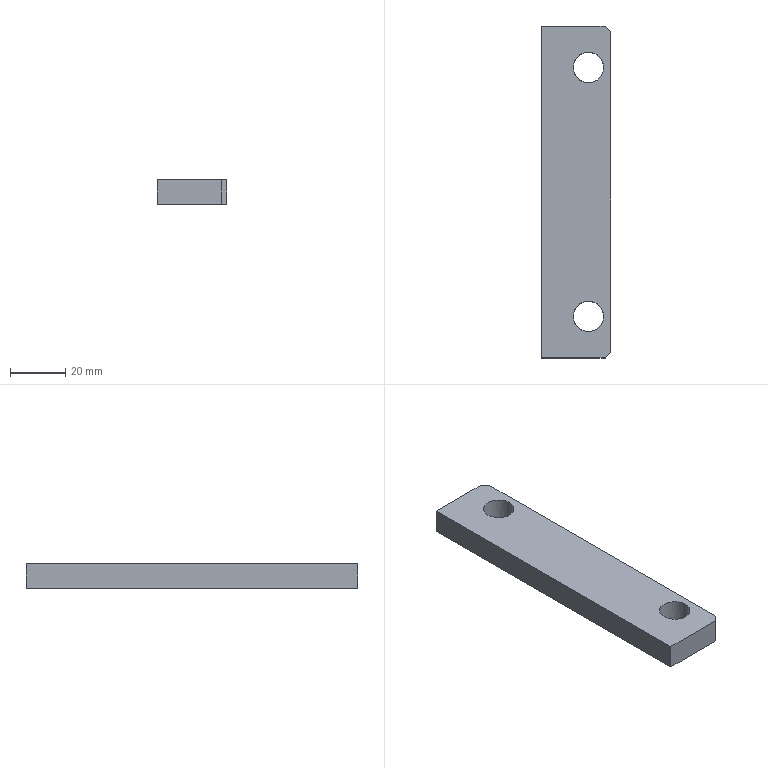Part | NX | features solid 2 | 1 solid | 10 faces | box 25 x 120 x 9 mm | volume 25253 mm3 | plane 8 | cylinder 2 | commonest cylinder face diameters 11 x2
STEP:
#1=CARTESIAN_POINT('',(59.5,685.,-99.));
#2=VERTEX_POINT('',#1);
#3=CARTESIAN_POINT('',(54.,685.,-99.));
#4=DIRECTION('',(0.,0.,1.));
#5=DIRECTION('',(1.,0.,0.));
#6=AXIS2_PLACEMENT_3D('',#3,#4,#5);
#7=CIRCLE('',#6,5.5);
#8=EDGE_CURVE('',#2,#2,#7,.F.);
#9=ORIENTED_EDGE('',*,*,#8,.T.);
#10=EDGE_LOOP('',(#9));
#11=FACE_BOUND('',#10,.T.);
#12=CARTESIAN_POINT('',(59.5,595.,-99.));
#13=VERTEX_POINT('',#12);
#14=CARTESIAN_POINT('',(54.,595.,-99.));
#15=DIRECTION('',(0.,0.,1.));
#16=DIRECTION('',(1.,0.,0.));
#17=AXIS2_PLACEMENT_3D('',#14,#15,#16);
#18=CIRCLE('',#17,5.5);
#19=EDGE_CURVE('',#13,#13,#18,.F.);
#20=ORIENTED_EDGE('',*,*,#19,.T.);
#21=EDGE_LOOP('',(#20));
#22=FACE_BOUND('',#21,.T.);
#23=CARTESIAN_POINT('',(62.,698.,-99.));
#24=VERTEX_POINT('',#23);
#25=CARTESIAN_POINT('',(62.,582.,-99.));
#26=VERTEX_POINT('',#25);
#27=CARTESIAN_POINT('',(62.,640.,-99.));
#28=DIRECTION('',(0.,-1.,0.));
#29=VECTOR('',#28,1000.);
#30=LINE('',#27,#29);
#31=EDGE_CURVE('',#24,#26,#30,.T.);
#32=ORIENTED_EDGE('',*,*,#31,.F.);
#33=CARTESIAN_POINT('',(60.,700.,-99.));
#34=VERTEX_POINT('',#33);
#35=CARTESIAN_POINT('',(84.75,675.25,-99.));
#36=DIRECTION('',(0.7071,-0.7071,0.));
#37=VECTOR('',#36,1000.);
#38=LINE('',#35,#37);
#39=EDGE_CURVE('',#24,#34,#38,.F.);
#40=ORIENTED_EDGE('',*,*,#39,.T.);
#41=CARTESIAN_POINT('',(37.,700.,-99.));
#42=VERTEX_POINT('',#41);
#43=CARTESIAN_POINT('',(49.5,700.,-99.));
#44=DIRECTION('',(1.,0.,0.));
#45=VECTOR('',#44,1000.);
#46=LINE('',#43,#45);
#47=EDGE_CURVE('',#42,#34,#46,.T.);
#48=ORIENTED_EDGE('',*,*,#47,.F.);
#49=CARTESIAN_POINT('',(37.,580.,-99.));
#50=VERTEX_POINT('',#49);
#51=CARTESIAN_POINT('',(37.,640.,-99.));
#52=DIRECTION('',(0.,1.,0.));
#53=VECTOR('',#52,1000.);
#54=LINE('',#51,#53);
#55=EDGE_CURVE('',#50,#42,#54,.T.);
#56=ORIENTED_EDGE('',*,*,#55,.F.);
#57=CARTESIAN_POINT('',(60.,580.,-99.));
#58=VERTEX_POINT('',#57);
#59=CARTESIAN_POINT('',(49.5,580.,-99.));
#60=DIRECTION('',(-1.,0.,0.));
#61=VECTOR('',#60,1000.);
#62=LINE('',#59,#61);
#63=EDGE_CURVE('',#58,#50,#62,.T.);
#64=ORIENTED_EDGE('',*,*,#63,.F.);
#65=CARTESIAN_POINT('',(84.75,604.75,-99.));
#66=DIRECTION('',(-0.7071,-0.7071,0.));
#67=VECTOR('',#66,1000.);
#68=LINE('',#65,#67);
#69=EDGE_CURVE('',#58,#26,#68,.F.);
#70=ORIENTED_EDGE('',*,*,#69,.T.);
#71=EDGE_LOOP('',(#32,#40,#48,#56,#64,#70));
#72=FACE_BOUND('',#71,.T.);
#73=CARTESIAN_POINT('',(49.5,640.,-99.));
#74=DIRECTION('',(0.,0.,1.));
#75=DIRECTION('',(0.,1.,0.));
#76=AXIS2_PLACEMENT_3D('',#73,#74,#75);
#77=PLANE('',#76);
#78=ADVANCED_FACE('',(#11,#22,#72),#77,.T.);
#79=CARTESIAN_POINT('',(62.,582.,-108.));
#80=VERTEX_POINT('',#79);
#81=CARTESIAN_POINT('',(62.,698.,-108.));
#82=VERTEX_POINT('',#81);
#83=CARTESIAN_POINT('',(62.,640.,-108.));
#84=DIRECTION('',(0.,1.,0.));
#85=VECTOR('',#84,1000.);
#86=LINE('',#83,#85);
#87=EDGE_CURVE('',#80,#82,#86,.T.);
#88=ORIENTED_EDGE('',*,*,#87,.T.);
#89=CARTESIAN_POINT('',(62.,698.,-108.));
#90=DIRECTION('',(0.,0.,1.));
#91=VECTOR('',#90,1000.);
#92=LINE('',#89,#91);
#93=EDGE_CURVE('',#82,#24,#92,.T.);
#94=ORIENTED_EDGE('',*,*,#93,.T.);
#95=ORIENTED_EDGE('',*,*,#31,.T.);
#96=CARTESIAN_POINT('',(62.,582.,-108.));
#97=DIRECTION('',(0.,0.,-1.));
#98=VECTOR('',#97,1000.);
#99=LINE('',#96,#98);
#100=EDGE_CURVE('',#26,#80,#99,.T.);
#101=ORIENTED_EDGE('',*,*,#100,.T.);
#102=EDGE_LOOP('',(#88,#94,#95,#101));
#103=FACE_BOUND('',#102,.T.);
#104=CARTESIAN_POINT('',(62.,640.,-108.));
#105=DIRECTION('',(1.,0.,0.));
#106=DIRECTION('',(0.,0.,-1.));
#107=AXIS2_PLACEMENT_3D('',#104,#105,#106);
#108=PLANE('',#107);
#109=ADVANCED_FACE('',(#103),#108,.T.);
#110=CARTESIAN_POINT('',(37.,580.,-108.));
#111=VERTEX_POINT('',#110);
#112=CARTESIAN_POINT('',(60.,580.,-108.));
#113=VERTEX_POINT('',#112);
#114=CARTESIAN_POINT('',(49.5,580.,-108.));
#115=DIRECTION('',(1.,0.,0.));
#116=VECTOR('',#115,1000.);
#117=LINE('',#114,#116);
#118=EDGE_CURVE('',#111,#113,#117,.T.);
#119=ORIENTED_EDGE('',*,*,#118,.T.);
#120=CARTESIAN_POINT('',(60.,580.,-108.));
#121=DIRECTION('',(0.,0.,1.));
#122=VECTOR('',#121,1000.);
#123=LINE('',#120,#122);
#124=EDGE_CURVE('',#113,#58,#123,.T.);
#125=ORIENTED_EDGE('',*,*,#124,.T.);
#126=ORIENTED_EDGE('',*,*,#63,.T.);
#127=CARTESIAN_POINT('',(37.,580.,-108.));
#128=DIRECTION('',(0.,0.,1.));
#129=VECTOR('',#128,1000.);
#130=LINE('',#127,#129);
#131=EDGE_CURVE('',#111,#50,#130,.T.);
#132=ORIENTED_EDGE('',*,*,#131,.F.);
#133=EDGE_LOOP('',(#119,#125,#126,#132));
#134=FACE_BOUND('',#133,.T.);
#135=CARTESIAN_POINT('',(49.5,580.,-108.));
#136=DIRECTION('',(0.,-1.,0.));
#137=DIRECTION('',(0.,0.,1.));
#138=AXIS2_PLACEMENT_3D('',#135,#136,#137);
#139=PLANE('',#138);
#140=ADVANCED_FACE('',(#134),#139,.T.);
#141=ORIENTED_EDGE('',*,*,#131,.T.);
#142=ORIENTED_EDGE('',*,*,#55,.T.);
#143=CARTESIAN_POINT('',(37.,700.,-108.));
#144=VERTEX_POINT('',#143);
#145=CARTESIAN_POINT('',(37.,700.,-108.));
#146=DIRECTION('',(0.,0.,1.));
#147=VECTOR('',#146,1000.);
#148=LINE('',#145,#147);
#149=EDGE_CURVE('',#144,#42,#148,.T.);
#150=ORIENTED_EDGE('',*,*,#149,.F.);
#151=CARTESIAN_POINT('',(37.,640.,-108.));
#152=DIRECTION('',(0.,-1.,0.));
#153=VECTOR('',#152,1000.);
#154=LINE('',#151,#153);
#155=EDGE_CURVE('',#144,#111,#154,.T.);
#156=ORIENTED_EDGE('',*,*,#155,.T.);
#157=EDGE_LOOP('',(#141,#142,#150,#156));
#158=FACE_BOUND('',#157,.T.);
#159=CARTESIAN_POINT('',(37.,640.,-108.));
#160=DIRECTION('',(-1.,0.,0.));
#161=DIRECTION('',(0.,0.,1.));
#162=AXIS2_PLACEMENT_3D('',#159,#160,#161);
#163=PLANE('',#162);
#164=ADVANCED_FACE('',(#158),#163,.T.);
#165=CARTESIAN_POINT('',(54.,690.5,-108.));
#166=VERTEX_POINT('',#165);
#167=CARTESIAN_POINT('',(54.,685.,-108.));
#168=DIRECTION('',(0.,0.,-1.));
#169=DIRECTION('',(0.,1.,0.));
#170=AXIS2_PLACEMENT_3D('',#167,#168,#169);
#171=CIRCLE('',#170,5.5);
#172=EDGE_CURVE('',#166,#166,#171,.T.);
#173=ORIENTED_EDGE('',*,*,#172,.F.);
#174=EDGE_LOOP('',(#173));
#175=FACE_BOUND('',#174,.T.);
#176=CARTESIAN_POINT('',(54.,600.5,-108.));
#177=VERTEX_POINT('',#176);
#178=CARTESIAN_POINT('',(54.,595.,-108.));
#179=DIRECTION('',(0.,0.,-1.));
#180=DIRECTION('',(0.,1.,0.));
#181=AXIS2_PLACEMENT_3D('',#178,#179,#180);
#182=CIRCLE('',#181,5.5);
#183=EDGE_CURVE('',#177,#177,#182,.T.);
#184=ORIENTED_EDGE('',*,*,#183,.F.);
#185=EDGE_LOOP('',(#184));
#186=FACE_BOUND('',#185,.T.);
#187=CARTESIAN_POINT('',(60.,700.,-108.));
#188=VERTEX_POINT('',#187);
#189=CARTESIAN_POINT('',(49.5,700.,-108.));
#190=DIRECTION('',(-1.,0.,0.));
#191=VECTOR('',#190,1000.);
#192=LINE('',#189,#191);
#193=EDGE_CURVE('',#188,#144,#192,.T.);
#194=ORIENTED_EDGE('',*,*,#193,.F.);
#195=CARTESIAN_POINT('',(84.75,675.25,-108.));
#196=DIRECTION('',(-0.7071,0.7071,0.));
#197=VECTOR('',#196,1000.);
#198=LINE('',#195,#197);
#199=EDGE_CURVE('',#188,#82,#198,.F.);
#200=ORIENTED_EDGE('',*,*,#199,.T.);
#201=ORIENTED_EDGE('',*,*,#87,.F.);
#202=CARTESIAN_POINT('',(84.75,604.75,-108.));
#203=DIRECTION('',(0.7071,0.7071,0.));
#204=VECTOR('',#203,1000.);
#205=LINE('',#202,#204);
#206=EDGE_CURVE('',#80,#113,#205,.F.);
#207=ORIENTED_EDGE('',*,*,#206,.T.);
#208=ORIENTED_EDGE('',*,*,#118,.F.);
#209=ORIENTED_EDGE('',*,*,#155,.F.);
#210=EDGE_LOOP('',(#194,#200,#201,#207,#208,#209));
#211=FACE_BOUND('',#210,.T.);
#212=CARTESIAN_POINT('',(49.5,640.,-108.));
#213=DIRECTION('',(0.,0.,-1.));
#214=DIRECTION('',(0.,-1.,0.));
#215=AXIS2_PLACEMENT_3D('',#212,#213,#214);
#216=PLANE('',#215);
#217=ADVANCED_FACE('',(#175,#186,#211),#216,.T.);
#218=ORIENTED_EDGE('',*,*,#47,.T.);
#219=CARTESIAN_POINT('',(60.,700.,-108.));
#220=DIRECTION('',(0.,0.,-1.));
#221=VECTOR('',#220,1000.);
#222=LINE('',#219,#221);
#223=EDGE_CURVE('',#34,#188,#222,.T.);
#224=ORIENTED_EDGE('',*,*,#223,.T.);
#225=ORIENTED_EDGE('',*,*,#193,.T.);
#226=ORIENTED_EDGE('',*,*,#149,.T.);
#227=EDGE_LOOP('',(#218,#224,#225,#226));
#228=FACE_BOUND('',#227,.T.);
#229=CARTESIAN_POINT('',(49.5,700.,-108.));
#230=DIRECTION('',(0.,1.,0.));
#231=DIRECTION('',(0.,0.,-1.));
#232=AXIS2_PLACEMENT_3D('',#229,#230,#231);
#233=PLANE('',#232);
#234=ADVANCED_FACE('',(#228),#233,.T.);
#235=ORIENTED_EDGE('',*,*,#183,.T.);
#236=EDGE_LOOP('',(#235));
#237=FACE_BOUND('',#236,.T.);
#238=ORIENTED_EDGE('',*,*,#19,.F.);
#239=EDGE_LOOP('',(#238));
#240=FACE_BOUND('',#239,.T.);
#241=CARTESIAN_POINT('',(54.,595.,-98.));
#242=DIRECTION('',(0.,0.,-1.));
#243=DIRECTION('',(0.,-1.,0.));
#244=AXIS2_PLACEMENT_3D('',#241,#242,#243);
#245=CYLINDRICAL_SURFACE('',#244,5.5);
#246=ADVANCED_FACE('',(#237,#240),#245,.F.);
#247=ORIENTED_EDGE('',*,*,#172,.T.);
#248=EDGE_LOOP('',(#247));
#249=FACE_BOUND('',#248,.T.);
#250=ORIENTED_EDGE('',*,*,#8,.F.);
#251=EDGE_LOOP('',(#250));
#252=FACE_BOUND('',#251,.T.);
#253=CARTESIAN_POINT('',(54.,685.,-98.));
#254=DIRECTION('',(0.,0.,-1.));
#255=DIRECTION('',(0.,-1.,0.));
#256=AXIS2_PLACEMENT_3D('',#253,#254,#255);
#257=CYLINDRICAL_SURFACE('',#256,5.5);
#258=ADVANCED_FACE('',(#249,#252),#257,.F.);
#259=ORIENTED_EDGE('',*,*,#199,.F.);
#260=ORIENTED_EDGE('',*,*,#223,.F.);
#261=ORIENTED_EDGE('',*,*,#39,.F.);
#262=ORIENTED_EDGE('',*,*,#93,.F.);
#263=EDGE_LOOP('',(#259,#260,#261,#262));
#264=FACE_BOUND('',#263,.T.);
#265=CARTESIAN_POINT('',(62.,698.,-108.));
#266=DIRECTION('',(-0.7071,-0.7071,0.));
#267=DIRECTION('',(0.7071,-0.7071,0.));
#268=AXIS2_PLACEMENT_3D('',#265,#266,#267);
#269=PLANE('',#268);
#270=ADVANCED_FACE('',(#264),#269,.F.);
#271=ORIENTED_EDGE('',*,*,#206,.F.);
#272=ORIENTED_EDGE('',*,*,#100,.F.);
#273=ORIENTED_EDGE('',*,*,#69,.F.);
#274=ORIENTED_EDGE('',*,*,#124,.F.);
#275=EDGE_LOOP('',(#271,#272,#273,#274));
#276=FACE_BOUND('',#275,.T.);
#277=CARTESIAN_POINT('',(60.,580.,-108.));
#278=DIRECTION('',(-0.7071,0.7071,0.));
#279=DIRECTION('',(-0.7071,-0.7071,0.));
#280=AXIS2_PLACEMENT_3D('',#277,#278,#279);
#281=PLANE('',#280);
#282=ADVANCED_FACE('',(#276),#281,.F.);
#283=CLOSED_SHELL('',(#78,#109,#140,#164,#217,#234,#246,#258,#270,#282));
#284=MANIFOLD_SOLID_BREP('',#283);
#285=(LENGTH_UNIT()NAMED_UNIT(*)SI_UNIT(.MILLI.,.METRE.));
#286=UNCERTAINTY_MEASURE_WITH_UNIT(LENGTH_MEASURE(0.00001),#285,'','');
#287=(NAMED_UNIT(*)PLANE_ANGLE_UNIT()SI_UNIT($,.RADIAN.));
#288=(NAMED_UNIT(*)SI_UNIT($,.STERADIAN.)SOLID_ANGLE_UNIT());
#289=(GEOMETRIC_REPRESENTATION_CONTEXT(3)GLOBAL_UNCERTAINTY_ASSIGNED_CONTEXT((#286))GLOBAL_UNIT_ASSIGNED_CONTEXT((#285,#287,#288))REPRESENTATION_CONTEXT('',''));
#290=ADVANCED_BREP_SHAPE_REPRESENTATION('',(#284),#289);